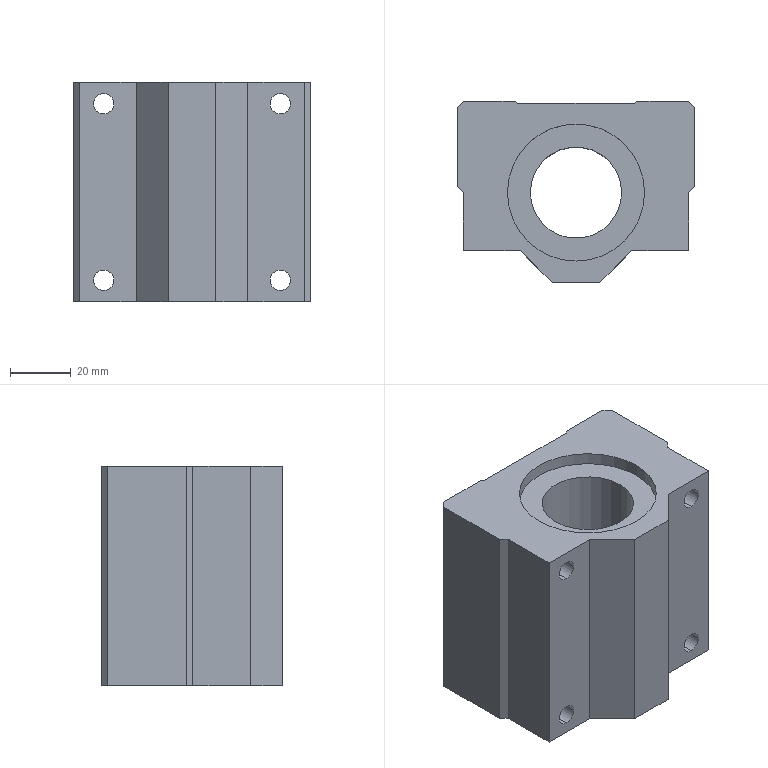Part | SolidWorks | features MBimport 1 | 1 solid | 44 faces | box 78 x 59.5 x 72 mm | volume 221969 mm3 | plane 22 | cylinder 14 | cone 8 | commonest cylinder face diameters 6.647 x8 45 x4 30 x2
STEP:
#1=CARTESIAN_POINT('',(-29.,29.324,-68.323));
#2=VERTEX_POINT('',#1);
#3=CARTESIAN_POINT('',(-29.,29.324,-61.676));
#4=VERTEX_POINT('',#3);
#5=CARTESIAN_POINT('',(-29.,29.324,-65.));
#6=DIRECTION('',(0.,1.,0.));
#7=DIRECTION('',(0.,0.,1.));
#8=AXIS2_PLACEMENT_3D('',#5,#6,#7);
#9=CIRCLE('',#8,3.323);
#10=EDGE_CURVE('',#2,#4,#9,.T.);
#11=ORIENTED_EDGE('',*,*,#10,.F.);
#12=CARTESIAN_POINT('',(-29.,30.,-69.));
#13=VERTEX_POINT('',#12);
#14=CARTESIAN_POINT('',(-29.,29.324,-68.323));
#15=DIRECTION('',(0.,0.7071,-0.7071));
#16=VECTOR('',#15,1000.);
#17=LINE('',#14,#16);
#18=EDGE_CURVE('',#2,#13,#17,.T.);
#19=ORIENTED_EDGE('',*,*,#18,.T.);
#20=CARTESIAN_POINT('',(-29.,30.,-61.));
#21=VERTEX_POINT('',#20);
#22=CARTESIAN_POINT('',(-29.,30.,-65.));
#23=DIRECTION('',(0.,1.,0.));
#24=DIRECTION('',(0.,0.,1.));
#25=AXIS2_PLACEMENT_3D('',#22,#23,#24);
#26=CIRCLE('',#25,4.);
#27=EDGE_CURVE('',#13,#21,#26,.T.);
#28=ORIENTED_EDGE('',*,*,#27,.T.);
#29=CARTESIAN_POINT('',(-29.,29.324,-61.676));
#30=DIRECTION('',(0.,0.7071,0.7071));
#31=VECTOR('',#30,1000.);
#32=LINE('',#29,#31);
#33=EDGE_CURVE('',#4,#21,#32,.T.);
#34=ORIENTED_EDGE('',*,*,#33,.F.);
#35=EDGE_LOOP('',(#11,#19,#28,#34));
#36=FACE_OUTER_BOUND('',#35,.T.);
#37=CARTESIAN_POINT('',(-29.,29.324,-65.));
#38=DIRECTION('',(0.,1.,0.));
#39=DIRECTION('',(0.,0.,1.));
#40=AXIS2_PLACEMENT_3D('',#37,#38,#39);
#41=CONICAL_SURFACE('',#40,3.323,0.7854);
#42=ADVANCED_FACE('',(#36),#41,.F.);
#43=CARTESIAN_POINT('',(-29.,29.324,-65.));
#44=DIRECTION('',(0.,1.,0.));
#45=DIRECTION('',(0.,0.,1.));
#46=AXIS2_PLACEMENT_3D('',#43,#44,#45);
#47=CIRCLE('',#46,3.323);
#48=EDGE_CURVE('',#4,#2,#47,.T.);
#49=ORIENTED_EDGE('',*,*,#48,.T.);
#50=CARTESIAN_POINT('',(-29.,-19.,-68.324));
#51=VERTEX_POINT('',#50);
#52=CARTESIAN_POINT('',(-29.,30.,-68.323));
#53=DIRECTION('',(0.,-1.,0.));
#54=VECTOR('',#53,1000.);
#55=LINE('',#52,#54);
#56=EDGE_CURVE('',#2,#51,#55,.T.);
#57=ORIENTED_EDGE('',*,*,#56,.T.);
#58=CARTESIAN_POINT('',(-29.,-19.,-61.677));
#59=VERTEX_POINT('',#58);
#60=CARTESIAN_POINT('',(-29.,-19.,-65.));
#61=DIRECTION('',(0.,1.,0.));
#62=DIRECTION('',(0.,0.,1.));
#63=AXIS2_PLACEMENT_3D('',#60,#61,#62);
#64=CIRCLE('',#63,3.323);
#65=EDGE_CURVE('',#59,#51,#64,.T.);
#66=ORIENTED_EDGE('',*,*,#65,.F.);
#67=CARTESIAN_POINT('',(-29.,30.,-61.676));
#68=DIRECTION('',(0.,-1.,0.));
#69=VECTOR('',#68,1000.);
#70=LINE('',#67,#69);
#71=EDGE_CURVE('',#4,#59,#70,.T.);
#72=ORIENTED_EDGE('',*,*,#71,.F.);
#73=EDGE_LOOP('',(#49,#57,#66,#72));
#74=FACE_OUTER_BOUND('',#73,.T.);
#75=CARTESIAN_POINT('',(-29.,30.,-65.));
#76=DIRECTION('',(0.,-1.,0.));
#77=DIRECTION('',(0.,0.,1.));
#78=AXIS2_PLACEMENT_3D('',#75,#76,#77);
#79=CYLINDRICAL_SURFACE('',#78,3.323);
#80=ADVANCED_FACE('',(#74),#79,.F.);
#81=CARTESIAN_POINT('',(29.,-19.,-68.324));
#82=VERTEX_POINT('',#81);
#83=CARTESIAN_POINT('',(29.,-19.,-61.677));
#84=VERTEX_POINT('',#83);
#85=CARTESIAN_POINT('',(29.,-19.,-65.));
#86=DIRECTION('',(0.,-1.,0.));
#87=DIRECTION('',(0.,0.,-1.));
#88=AXIS2_PLACEMENT_3D('',#85,#86,#87);
#89=CIRCLE('',#88,3.323);
#90=EDGE_CURVE('',#82,#84,#89,.T.);
#91=ORIENTED_EDGE('',*,*,#90,.T.);
#92=CARTESIAN_POINT('',(29.,29.324,-61.677));
#93=VERTEX_POINT('',#92);
#94=CARTESIAN_POINT('',(29.,-19.,-61.677));
#95=DIRECTION('',(0.,1.,0.));
#96=VECTOR('',#95,1000.);
#97=LINE('',#94,#96);
#98=EDGE_CURVE('',#84,#93,#97,.T.);
#99=ORIENTED_EDGE('',*,*,#98,.T.);
#100=CARTESIAN_POINT('',(29.,29.324,-68.324));
#101=VERTEX_POINT('',#100);
#102=CARTESIAN_POINT('',(29.,29.324,-65.));
#103=DIRECTION('',(0.,-1.,0.));
#104=DIRECTION('',(0.,0.,-1.));
#105=AXIS2_PLACEMENT_3D('',#102,#103,#104);
#106=CIRCLE('',#105,3.323);
#107=EDGE_CURVE('',#101,#93,#106,.T.);
#108=ORIENTED_EDGE('',*,*,#107,.F.);
#109=CARTESIAN_POINT('',(29.,-19.,-68.324));
#110=DIRECTION('',(0.,1.,0.));
#111=VECTOR('',#110,1000.);
#112=LINE('',#109,#111);
#113=EDGE_CURVE('',#82,#101,#112,.T.);
#114=ORIENTED_EDGE('',*,*,#113,.F.);
#115=EDGE_LOOP('',(#91,#99,#108,#114));
#116=FACE_OUTER_BOUND('',#115,.T.);
#117=CARTESIAN_POINT('',(29.,-19.,-65.));
#118=DIRECTION('',(0.,1.,0.));
#119=DIRECTION('',(0.,0.,-1.));
#120=AXIS2_PLACEMENT_3D('',#117,#118,#119);
#121=CYLINDRICAL_SURFACE('',#120,3.323);
#122=ADVANCED_FACE('',(#116),#121,.F.);
#123=CARTESIAN_POINT('',(29.,29.324,-65.));
#124=DIRECTION('',(0.,-1.,0.));
#125=DIRECTION('',(0.,0.,-1.));
#126=AXIS2_PLACEMENT_3D('',#123,#124,#125);
#127=CIRCLE('',#126,3.323);
#128=EDGE_CURVE('',#93,#101,#127,.T.);
#129=ORIENTED_EDGE('',*,*,#128,.T.);
#130=CARTESIAN_POINT('',(29.,30.,-69.));
#131=VERTEX_POINT('',#130);
#132=CARTESIAN_POINT('',(29.,30.,-69.));
#133=DIRECTION('',(0.,0.7071,-0.7071));
#134=VECTOR('',#133,1000.);
#135=LINE('',#132,#134);
#136=EDGE_CURVE('',#101,#131,#135,.T.);
#137=ORIENTED_EDGE('',*,*,#136,.T.);
#138=CARTESIAN_POINT('',(29.,30.,-61.));
#139=VERTEX_POINT('',#138);
#140=CARTESIAN_POINT('',(29.,30.,-65.));
#141=DIRECTION('',(0.,-1.,0.));
#142=DIRECTION('',(0.,0.,-1.));
#143=AXIS2_PLACEMENT_3D('',#140,#141,#142);
#144=CIRCLE('',#143,4.);
#145=EDGE_CURVE('',#139,#131,#144,.T.);
#146=ORIENTED_EDGE('',*,*,#145,.F.);
#147=CARTESIAN_POINT('',(29.,30.,-61.));
#148=DIRECTION('',(0.,0.7071,0.7071));
#149=VECTOR('',#148,1000.);
#150=LINE('',#147,#149);
#151=EDGE_CURVE('',#93,#139,#150,.T.);
#152=ORIENTED_EDGE('',*,*,#151,.F.);
#153=EDGE_LOOP('',(#129,#137,#146,#152));
#154=FACE_OUTER_BOUND('',#153,.T.);
#155=CARTESIAN_POINT('',(29.,30.,-65.));
#156=DIRECTION('',(0.,1.,0.));
#157=DIRECTION('',(0.,0.,1.));
#158=AXIS2_PLACEMENT_3D('',#155,#156,#157);
#159=CONICAL_SURFACE('',#158,4.,0.7854);
#160=ADVANCED_FACE('',(#154),#159,.F.);
#161=CARTESIAN_POINT('',(-29.,29.324,-10.323));
#162=VERTEX_POINT('',#161);
#163=CARTESIAN_POINT('',(-29.,29.324,-3.676));
#164=VERTEX_POINT('',#163);
#165=CARTESIAN_POINT('',(-29.,29.324,-7.));
#166=DIRECTION('',(0.,1.,0.));
#167=DIRECTION('',(0.,0.,1.));
#168=AXIS2_PLACEMENT_3D('',#165,#166,#167);
#169=CIRCLE('',#168,3.323);
#170=EDGE_CURVE('',#162,#164,#169,.T.);
#171=ORIENTED_EDGE('',*,*,#170,.F.);
#172=CARTESIAN_POINT('',(-29.,30.,-11.));
#173=VERTEX_POINT('',#172);
#174=CARTESIAN_POINT('',(-29.,29.324,-10.323));
#175=DIRECTION('',(0.,0.7071,-0.7071));
#176=VECTOR('',#175,1000.);
#177=LINE('',#174,#176);
#178=EDGE_CURVE('',#162,#173,#177,.T.);
#179=ORIENTED_EDGE('',*,*,#178,.T.);
#180=CARTESIAN_POINT('',(-29.,30.,-3.));
#181=VERTEX_POINT('',#180);
#182=CARTESIAN_POINT('',(-29.,30.,-7.));
#183=DIRECTION('',(0.,1.,0.));
#184=DIRECTION('',(0.,0.,1.));
#185=AXIS2_PLACEMENT_3D('',#182,#183,#184);
#186=CIRCLE('',#185,4.);
#187=EDGE_CURVE('',#173,#181,#186,.T.);
#188=ORIENTED_EDGE('',*,*,#187,.T.);
#189=CARTESIAN_POINT('',(-29.,29.324,-3.676));
#190=DIRECTION('',(0.,0.7071,0.7071));
#191=VECTOR('',#190,1000.);
#192=LINE('',#189,#191);
#193=EDGE_CURVE('',#164,#181,#192,.T.);
#194=ORIENTED_EDGE('',*,*,#193,.F.);
#195=EDGE_LOOP('',(#171,#179,#188,#194));
#196=FACE_OUTER_BOUND('',#195,.T.);
#197=CARTESIAN_POINT('',(-29.,29.324,-7.));
#198=DIRECTION('',(0.,1.,0.));
#199=DIRECTION('',(0.,0.,1.));
#200=AXIS2_PLACEMENT_3D('',#197,#198,#199);
#201=CONICAL_SURFACE('',#200,3.323,0.7854);
#202=ADVANCED_FACE('',(#196),#201,.F.);
#203=CARTESIAN_POINT('',(-22.5,0.,-72.));
#204=VERTEX_POINT('',#203);
#205=CARTESIAN_POINT('',(22.5,0.,-72.));
#206=VERTEX_POINT('',#205);
#207=CARTESIAN_POINT('',(0.,0.,-72.));
#208=DIRECTION('',(0.,0.,-1.));
#209=DIRECTION('',(-1.,0.,0.));
#210=AXIS2_PLACEMENT_3D('',#207,#208,#209);
#211=CIRCLE('',#210,22.5);
#212=EDGE_CURVE('',#204,#206,#211,.T.);
#213=ORIENTED_EDGE('',*,*,#212,.T.);
#214=CARTESIAN_POINT('',(22.5,0.,-68.));
#215=VERTEX_POINT('',#214);
#216=CARTESIAN_POINT('',(22.5,0.,-72.));
#217=DIRECTION('',(0.,0.,1.));
#218=VECTOR('',#217,1000.);
#219=LINE('',#216,#218);
#220=EDGE_CURVE('',#206,#215,#219,.T.);
#221=ORIENTED_EDGE('',*,*,#220,.T.);
#222=CARTESIAN_POINT('',(-22.5,0.,-68.));
#223=VERTEX_POINT('',#222);
#224=CARTESIAN_POINT('',(0.,0.,-68.));
#225=DIRECTION('',(0.,0.,-1.));
#226=DIRECTION('',(-1.,0.,0.));
#227=AXIS2_PLACEMENT_3D('',#224,#225,#226);
#228=CIRCLE('',#227,22.5);
#229=EDGE_CURVE('',#223,#215,#228,.T.);
#230=ORIENTED_EDGE('',*,*,#229,.F.);
#231=CARTESIAN_POINT('',(-22.5,0.,-72.));
#232=DIRECTION('',(0.,0.,1.));
#233=VECTOR('',#232,1000.);
#234=LINE('',#231,#233);
#235=EDGE_CURVE('',#204,#223,#234,.T.);
#236=ORIENTED_EDGE('',*,*,#235,.F.);
#237=EDGE_LOOP('',(#213,#221,#230,#236));
#238=FACE_OUTER_BOUND('',#237,.T.);
#239=CARTESIAN_POINT('',(0.,0.,-72.));
#240=DIRECTION('',(0.,0.,1.));
#241=DIRECTION('',(-1.,0.,0.));
#242=AXIS2_PLACEMENT_3D('',#239,#240,#241);
#243=CYLINDRICAL_SURFACE('',#242,22.5);
#244=ADVANCED_FACE('',(#238),#243,.F.);
#245=CARTESIAN_POINT('',(29.,29.324,-3.677));
#246=VERTEX_POINT('',#245);
#247=CARTESIAN_POINT('',(29.,29.324,-10.323));
#248=VERTEX_POINT('',#247);
#249=CARTESIAN_POINT('',(29.,29.324,-7.));
#250=DIRECTION('',(0.,-1.,0.));
#251=DIRECTION('',(0.,0.,-1.));
#252=AXIS2_PLACEMENT_3D('',#249,#250,#251);
#253=CIRCLE('',#252,3.323);
#254=EDGE_CURVE('',#246,#248,#253,.T.);
#255=ORIENTED_EDGE('',*,*,#254,.T.);
#256=CARTESIAN_POINT('',(29.,30.,-11.));
#257=VERTEX_POINT('',#256);
#258=CARTESIAN_POINT('',(29.,30.,-11.));
#259=DIRECTION('',(0.,0.7071,-0.7071));
#260=VECTOR('',#259,1000.);
#261=LINE('',#258,#260);
#262=EDGE_CURVE('',#248,#257,#261,.T.);
#263=ORIENTED_EDGE('',*,*,#262,.T.);
#264=CARTESIAN_POINT('',(29.,30.,-3.));
#265=VERTEX_POINT('',#264);
#266=CARTESIAN_POINT('',(29.,30.,-7.));
#267=DIRECTION('',(0.,-1.,0.));
#268=DIRECTION('',(0.,0.,-1.));
#269=AXIS2_PLACEMENT_3D('',#266,#267,#268);
#270=CIRCLE('',#269,4.);
#271=EDGE_CURVE('',#265,#257,#270,.T.);
#272=ORIENTED_EDGE('',*,*,#271,.F.);
#273=CARTESIAN_POINT('',(29.,30.,-3.));
#274=DIRECTION('',(0.,0.7071,0.7071));
#275=VECTOR('',#274,1000.);
#276=LINE('',#273,#275);
#277=EDGE_CURVE('',#246,#265,#276,.T.);
#278=ORIENTED_EDGE('',*,*,#277,.F.);
#279=EDGE_LOOP('',(#255,#263,#272,#278));
#280=FACE_OUTER_BOUND('',#279,.T.);
#281=CARTESIAN_POINT('',(29.,30.,-7.));
#282=DIRECTION('',(0.,1.,0.));
#283=DIRECTION('',(0.,0.,1.));
#284=AXIS2_PLACEMENT_3D('',#281,#282,#283);
#285=CONICAL_SURFACE('',#284,4.,0.7854);
#286=ADVANCED_FACE('',(#280),#285,.F.);
#287=CARTESIAN_POINT('',(-29.,29.324,-7.));
#288=DIRECTION('',(0.,1.,0.));
#289=DIRECTION('',(0.,0.,1.));
#290=AXIS2_PLACEMENT_3D('',#287,#288,#289);
#291=CIRCLE('',#290,3.323);
#292=EDGE_CURVE('',#164,#162,#291,.T.);
#293=ORIENTED_EDGE('',*,*,#292,.T.);
#294=CARTESIAN_POINT('',(-29.,-19.,-10.324));
#295=VERTEX_POINT('',#294);
#296=CARTESIAN_POINT('',(-29.,30.,-10.323));
#297=DIRECTION('',(0.,-1.,0.));
#298=VECTOR('',#297,1000.);
#299=LINE('',#296,#298);
#300=EDGE_CURVE('',#162,#295,#299,.T.);
#301=ORIENTED_EDGE('',*,*,#300,.T.);
#302=CARTESIAN_POINT('',(-29.,-19.,-3.677));
#303=VERTEX_POINT('',#302);
#304=CARTESIAN_POINT('',(-29.,-19.,-7.));
#305=DIRECTION('',(0.,1.,0.));
#306=DIRECTION('',(0.,0.,1.));
#307=AXIS2_PLACEMENT_3D('',#304,#305,#306);
#308=CIRCLE('',#307,3.323);
#309=EDGE_CURVE('',#303,#295,#308,.T.);
#310=ORIENTED_EDGE('',*,*,#309,.F.);
#311=CARTESIAN_POINT('',(-29.,30.,-3.676));
#312=DIRECTION('',(0.,-1.,0.));
#313=VECTOR('',#312,1000.);
#314=LINE('',#311,#313);
#315=EDGE_CURVE('',#164,#303,#314,.T.);
#316=ORIENTED_EDGE('',*,*,#315,.F.);
#317=EDGE_LOOP('',(#293,#301,#310,#316));
#318=FACE_OUTER_BOUND('',#317,.T.);
#319=CARTESIAN_POINT('',(-29.,30.,-7.));
#320=DIRECTION('',(0.,-1.,0.));
#321=DIRECTION('',(0.,0.,1.));
#322=AXIS2_PLACEMENT_3D('',#319,#320,#321);
#323=CYLINDRICAL_SURFACE('',#322,3.323);
#324=ADVANCED_FACE('',(#318),#323,.F.);
#325=CARTESIAN_POINT('',(29.,-19.,-10.324));
#326=VERTEX_POINT('',#325);
#327=CARTESIAN_POINT('',(29.,-19.,-3.677));
#328=VERTEX_POINT('',#327);
#329=CARTESIAN_POINT('',(29.,-19.,-7.));
#330=DIRECTION('',(0.,-1.,0.));
#331=DIRECTION('',(0.,0.,-1.));
#332=AXIS2_PLACEMENT_3D('',#329,#330,#331);
#333=CIRCLE('',#332,3.323);
#334=EDGE_CURVE('',#326,#328,#333,.T.);
#335=ORIENTED_EDGE('',*,*,#334,.T.);
#336=CARTESIAN_POINT('',(29.,-19.,-3.677));
#337=DIRECTION('',(0.,1.,0.));
#338=VECTOR('',#337,1000.);
#339=LINE('',#336,#338);
#340=EDGE_CURVE('',#328,#246,#339,.T.);
#341=ORIENTED_EDGE('',*,*,#340,.T.);
#342=CARTESIAN_POINT('',(29.,29.324,-7.));
#343=DIRECTION('',(0.,-1.,0.));
#344=DIRECTION('',(0.,0.,-1.));
#345=AXIS2_PLACEMENT_3D('',#342,#343,#344);
#346=CIRCLE('',#345,3.323);
#347=EDGE_CURVE('',#248,#246,#346,.T.);
#348=ORIENTED_EDGE('',*,*,#347,.F.);
#349=CARTESIAN_POINT('',(29.,-19.,-10.324));
#350=DIRECTION('',(0.,1.,0.));
#351=VECTOR('',#350,1000.);
#352=LINE('',#349,#351);
#353=EDGE_CURVE('',#326,#248,#352,.T.);
#354=ORIENTED_EDGE('',*,*,#353,.F.);
#355=EDGE_LOOP('',(#335,#341,#348,#354));
#356=FACE_OUTER_BOUND('',#355,.T.);
#357=CARTESIAN_POINT('',(29.,-19.,-7.));
#358=DIRECTION('',(0.,1.,0.));
#359=DIRECTION('',(0.,0.,-1.));
#360=AXIS2_PLACEMENT_3D('',#357,#358,#359);
#361=CYLINDRICAL_SURFACE('',#360,3.323);
#362=ADVANCED_FACE('',(#356),#361,.F.);
#363=CARTESIAN_POINT('',(-15.,0.,-68.));
#364=VERTEX_POINT('',#363);
#365=CARTESIAN_POINT('',(15.,0.,-68.));
#366=VERTEX_POINT('',#365);
#367=CARTESIAN_POINT('',(0.,0.,-68.));
#368=DIRECTION('',(0.,0.,-1.));
#369=DIRECTION('',(-1.,0.,0.));
#370=AXIS2_PLACEMENT_3D('',#367,#368,#369);
#371=CIRCLE('',#370,15.);
#372=EDGE_CURVE('',#364,#366,#371,.T.);
#373=ORIENTED_EDGE('',*,*,#372,.T.);
#374=CARTESIAN_POINT('',(15.,0.,-4.));
#375=VERTEX_POINT('',#374);
#376=CARTESIAN_POINT('',(15.,0.,-72.));
#377=DIRECTION('',(0.,0.,1.));
#378=VECTOR('',#377,1000.);
#379=LINE('',#376,#378);
#380=EDGE_CURVE('',#366,#375,#379,.T.);
#381=ORIENTED_EDGE('',*,*,#380,.T.);
#382=CARTESIAN_POINT('',(-15.,0.,-4.));
#383=VERTEX_POINT('',#382);
#384=CARTESIAN_POINT('',(0.,0.,-4.));
#385=DIRECTION('',(0.,0.,-1.));
#386=DIRECTION('',(-1.,0.,0.));
#387=AXIS2_PLACEMENT_3D('',#384,#385,#386);
#388=CIRCLE('',#387,15.);
#389=EDGE_CURVE('',#383,#375,#388,.T.);
#390=ORIENTED_EDGE('',*,*,#389,.F.);
#391=CARTESIAN_POINT('',(-15.,0.,-72.));
#392=DIRECTION('',(0.,0.,1.));
#393=VECTOR('',#392,1000.);
#394=LINE('',#391,#393);
#395=EDGE_CURVE('',#364,#383,#394,.T.);
#396=ORIENTED_EDGE('',*,*,#395,.F.);
#397=EDGE_LOOP('',(#373,#381,#390,#396));
#398=FACE_OUTER_BOUND('',#397,.T.);
#399=CARTESIAN_POINT('',(0.,0.,-72.));
#400=DIRECTION('',(0.,0.,1.));
#401=DIRECTION('',(-1.,0.,0.));
#402=AXIS2_PLACEMENT_3D('',#399,#400,#401);
#403=CYLINDRICAL_SURFACE('',#402,15.);
#404=ADVANCED_FACE('',(#398),#403,.F.);
#405=CARTESIAN_POINT('',(-22.5,0.,-4.));
#406=VERTEX_POINT('',#405);
#407=CARTESIAN_POINT('',(22.5,0.,-4.));
#408=VERTEX_POINT('',#407);
#409=CARTESIAN_POINT('',(0.,0.,-4.));
#410=DIRECTION('',(0.,0.,-1.));
#411=DIRECTION('',(-1.,0.,0.));
#412=AXIS2_PLACEMENT_3D('',#409,#410,#411);
#413=CIRCLE('',#412,22.5);
#414=EDGE_CURVE('',#406,#408,#413,.T.);
#415=ORIENTED_EDGE('',*,*,#414,.T.);
#416=CARTESIAN_POINT('',(22.5,0.,0.));
#417=VERTEX_POINT('',#416);
#418=CARTESIAN_POINT('',(22.5,0.,-72.));
#419=DIRECTION('',(0.,0.,1.));
#420=VECTOR('',#419,1000.);
#421=LINE('',#418,#420);
#422=EDGE_CURVE('',#408,#417,#421,.T.);
#423=ORIENTED_EDGE('',*,*,#422,.T.);
#424=CARTESIAN_POINT('',(-22.5,0.,0.));
#425=VERTEX_POINT('',#424);
#426=CARTESIAN_POINT('',(0.,0.,0.));
#427=DIRECTION('',(0.,0.,-1.));
#428=DIRECTION('',(-1.,0.,0.));
#429=AXIS2_PLACEMENT_3D('',#426,#427,#428);
#430=CIRCLE('',#429,22.5);
#431=EDGE_CURVE('',#425,#417,#430,.T.);
#432=ORIENTED_EDGE('',*,*,#431,.F.);
#433=CARTESIAN_POINT('',(-22.5,0.,-72.));
#434=DIRECTION('',(0.,0.,1.));
#435=VECTOR('',#434,1000.);
#436=LINE('',#433,#435);
#437=EDGE_CURVE('',#406,#425,#436,.T.);
#438=ORIENTED_EDGE('',*,*,#437,.F.);
#439=EDGE_LOOP('',(#415,#423,#432,#438));
#440=FACE_OUTER_BOUND('',#439,.T.);
#441=CARTESIAN_POINT('',(0.,0.,-72.));
#442=DIRECTION('',(0.,0.,1.));
#443=DIRECTION('',(-1.,0.,0.));
#444=AXIS2_PLACEMENT_3D('',#441,#442,#443);
#445=CYLINDRICAL_SURFACE('',#444,22.5);
#446=ADVANCED_FACE('',(#440),#445,.F.);
#447=CARTESIAN_POINT('',(-37.,-19.,0.));
#448=VERTEX_POINT('',#447);
#449=CARTESIAN_POINT('',(-18.3,-19.,0.));
#450=VERTEX_POINT('',#449);
#451=CARTESIAN_POINT('',(-37.,-19.,0.));
#452=DIRECTION('',(1.,0.,0.));
#453=VECTOR('',#452,1000.);
#454=LINE('',#451,#453);
#455=EDGE_CURVE('',#448,#450,#454,.T.);
#456=ORIENTED_EDGE('',*,*,#455,.F.);
#457=CARTESIAN_POINT('',(-37.,-19.,-72.));
#458=VERTEX_POINT('',#457);
#459=CARTESIAN_POINT('',(-37.,-19.,-72.));
#460=DIRECTION('',(0.,0.,1.));
#461=VECTOR('',#460,1000.);
#462=LINE('',#459,#461);
#463=EDGE_CURVE('',#458,#448,#462,.T.);
#464=ORIENTED_EDGE('',*,*,#463,.F.);
#465=CARTESIAN_POINT('',(-18.3,-19.,-72.));
#466=VERTEX_POINT('',#465);
#467=CARTESIAN_POINT('',(-37.,-19.,-72.));
#468=DIRECTION('',(1.,0.,0.));
#469=VECTOR('',#468,1000.);
#470=LINE('',#467,#469);
#471=EDGE_CURVE('',#458,#466,#470,.T.);
#472=ORIENTED_EDGE('',*,*,#471,.T.);
#473=CARTESIAN_POINT('',(-18.3,-19.,-72.));
#474=DIRECTION('',(0.,0.,1.));
#475=VECTOR('',#474,1000.);
#476=LINE('',#473,#475);
#477=EDGE_CURVE('',#466,#450,#476,.T.);
#478=ORIENTED_EDGE('',*,*,#477,.T.);
#479=EDGE_LOOP('',(#456,#464,#472,#478));
#480=FACE_OUTER_BOUND('',#479,.T.);
#481=ORIENTED_EDGE('',*,*,#309,.T.);
#482=CARTESIAN_POINT('',(-29.,-19.,-7.));
#483=DIRECTION('',(0.,1.,0.));
#484=DIRECTION('',(0.,0.,1.));
#485=AXIS2_PLACEMENT_3D('',#482,#483,#484);
#486=CIRCLE('',#485,3.323);
#487=EDGE_CURVE('',#295,#303,#486,.T.);
#488=ORIENTED_EDGE('',*,*,#487,.T.);
#489=EDGE_LOOP('',(#481,#488));
#490=FACE_BOUND('',#489,.T.);
#491=ORIENTED_EDGE('',*,*,#65,.T.);
#492=CARTESIAN_POINT('',(-29.,-19.,-65.));
#493=DIRECTION('',(0.,1.,0.));
#494=DIRECTION('',(0.,0.,1.));
#495=AXIS2_PLACEMENT_3D('',#492,#493,#494);
#496=CIRCLE('',#495,3.323);
#497=EDGE_CURVE('',#51,#59,#496,.T.);
#498=ORIENTED_EDGE('',*,*,#497,.T.);
#499=EDGE_LOOP('',(#491,#498));
#500=FACE_BOUND('',#499,.T.);
#501=CARTESIAN_POINT('',(-37.,-19.,-72.));
#502=DIRECTION('',(0.,-1.,0.));
#503=DIRECTION('',(0.,0.,-1.));
#504=AXIS2_PLACEMENT_3D('',#501,#502,#503);
#505=PLANE('',#504);
#506=ADVANCED_FACE('',(#480,#490,#500),#505,.T.);
#507=CARTESIAN_POINT('',(-39.,28.,0.));
#508=VERTEX_POINT('',#507);
#509=CARTESIAN_POINT('',(-39.,2.,0.));
#510=VERTEX_POINT('',#509);
#511=CARTESIAN_POINT('',(-39.,28.,0.));
#512=DIRECTION('',(0.,-1.,0.));
#513=VECTOR('',#512,1000.);
#514=LINE('',#511,#513);
#515=EDGE_CURVE('',#508,#510,#514,.T.);
#516=ORIENTED_EDGE('',*,*,#515,.F.);
#517=CARTESIAN_POINT('',(-39.,28.,-72.));
#518=VERTEX_POINT('',#517);
#519=CARTESIAN_POINT('',(-39.,28.,-72.));
#520=DIRECTION('',(0.,0.,1.));
#521=VECTOR('',#520,1000.);
#522=LINE('',#519,#521);
#523=EDGE_CURVE('',#518,#508,#522,.T.);
#524=ORIENTED_EDGE('',*,*,#523,.F.);
#525=CARTESIAN_POINT('',(-39.,2.,-72.));
#526=VERTEX_POINT('',#525);
#527=CARTESIAN_POINT('',(-39.,28.,-72.));
#528=DIRECTION('',(0.,-1.,0.));
#529=VECTOR('',#528,1000.);
#530=LINE('',#527,#529);
#531=EDGE_CURVE('',#518,#526,#530,.T.);
#532=ORIENTED_EDGE('',*,*,#531,.T.);
#533=CARTESIAN_POINT('',(-39.,2.,-72.));
#534=DIRECTION('',(0.,0.,1.));
#535=VECTOR('',#534,1000.);
#536=LINE('',#533,#535);
#537=EDGE_CURVE('',#526,#510,#536,.T.);
#538=ORIENTED_EDGE('',*,*,#537,.T.);
#539=EDGE_LOOP('',(#516,#524,#532,#538));
#540=FACE_OUTER_BOUND('',#539,.T.);
#541=CARTESIAN_POINT('',(-39.,28.,-72.));
#542=DIRECTION('',(-1.,0.,0.));
#543=DIRECTION('',(0.,0.,1.));
#544=AXIS2_PLACEMENT_3D('',#541,#542,#543);
#545=PLANE('',#544);
#546=ADVANCED_FACE('',(#540),#545,.T.);
#547=CARTESIAN_POINT('',(-19.95,30.,0.));
#548=VERTEX_POINT('',#547);
#549=CARTESIAN_POINT('',(-37.,30.,0.));
#550=VERTEX_POINT('',#549);
#551=CARTESIAN_POINT('',(-19.95,30.,0.));
#552=DIRECTION('',(-1.,0.,0.));
#553=VECTOR('',#552,1000.);
#554=LINE('',#551,#553);
#555=EDGE_CURVE('',#548,#550,#554,.T.);
#556=ORIENTED_EDGE('',*,*,#555,.F.);
#557=CARTESIAN_POINT('',(-19.95,30.,-72.));
#558=VERTEX_POINT('',#557);
#559=CARTESIAN_POINT('',(-19.95,30.,-72.));
#560=DIRECTION('',(0.,0.,1.));
#561=VECTOR('',#560,1000.);
#562=LINE('',#559,#561);
#563=EDGE_CURVE('',#558,#548,#562,.T.);
#564=ORIENTED_EDGE('',*,*,#563,.F.);
#565=CARTESIAN_POINT('',(-37.,30.,-72.));
#566=VERTEX_POINT('',#565);
#567=CARTESIAN_POINT('',(-19.95,30.,-72.));
#568=DIRECTION('',(-1.,0.,0.));
#569=VECTOR('',#568,1000.);
#570=LINE('',#567,#569);
#571=EDGE_CURVE('',#558,#566,#570,.T.);
#572=ORIENTED_EDGE('',*,*,#571,.T.);
#573=CARTESIAN_POINT('',(-37.,30.,-72.));
#574=DIRECTION('',(0.,0.,1.));
#575=VECTOR('',#574,1000.);
#576=LINE('',#573,#575);
#577=EDGE_CURVE('',#566,#550,#576,.T.);
#578=ORIENTED_EDGE('',*,*,#577,.T.);
#579=EDGE_LOOP('',(#556,#564,#572,#578));
#580=FACE_OUTER_BOUND('',#579,.T.);
#581=CARTESIAN_POINT('',(-29.,30.,-7.));
#582=DIRECTION('',(0.,1.,0.));
#583=DIRECTION('',(0.,0.,1.));
#584=AXIS2_PLACEMENT_3D('',#581,#582,#583);
#585=CIRCLE('',#584,4.);
#586=EDGE_CURVE('',#181,#173,#585,.T.);
#587=ORIENTED_EDGE('',*,*,#586,.F.);
#588=ORIENTED_EDGE('',*,*,#187,.F.);
#589=EDGE_LOOP('',(#587,#588));
#590=FACE_BOUND('',#589,.T.);
#591=CARTESIAN_POINT('',(-29.,30.,-65.));
#592=DIRECTION('',(0.,1.,0.));
#593=DIRECTION('',(0.,0.,1.));
#594=AXIS2_PLACEMENT_3D('',#591,#592,#593);
#595=CIRCLE('',#594,4.);
#596=EDGE_CURVE('',#21,#13,#595,.T.);
#597=ORIENTED_EDGE('',*,*,#596,.F.);
#598=ORIENTED_EDGE('',*,*,#27,.F.);
#599=EDGE_LOOP('',(#597,#598));
#600=FACE_BOUND('',#599,.T.);
#601=CARTESIAN_POINT('',(-19.95,30.,-72.));
#602=DIRECTION('',(0.,1.,0.));
#603=DIRECTION('',(1.,0.,0.));
#604=AXIS2_PLACEMENT_3D('',#601,#602,#603);
#605=PLANE('',#604);
#606=ADVANCED_FACE('',(#580,#590,#600),#605,.T.);
#607=CARTESIAN_POINT('',(-19.2,29.25,0.));
#608=VERTEX_POINT('',#607);
#609=CARTESIAN_POINT('',(-19.2,29.25,0.));
#610=DIRECTION('',(-0.7071,0.7071,0.));
#611=VECTOR('',#610,1000.);
#612=LINE('',#609,#611);
#613=EDGE_CURVE('',#608,#548,#612,.T.);
#614=ORIENTED_EDGE('',*,*,#613,.F.);
#615=CARTESIAN_POINT('',(-19.2,29.25,-72.));
#616=VERTEX_POINT('',#615);
#617=CARTESIAN_POINT('',(-19.2,29.25,-72.));
#618=DIRECTION('',(0.,0.,1.));
#619=VECTOR('',#618,1000.);
#620=LINE('',#617,#619);
#621=EDGE_CURVE('',#616,#608,#620,.T.);
#622=ORIENTED_EDGE('',*,*,#621,.F.);
#623=CARTESIAN_POINT('',(-19.2,29.25,-72.));
#624=DIRECTION('',(-0.7071,0.7071,0.));
#625=VECTOR('',#624,1000.);
#626=LINE('',#623,#625);
#627=EDGE_CURVE('',#616,#558,#626,.T.);
#628=ORIENTED_EDGE('',*,*,#627,.T.);
#629=ORIENTED_EDGE('',*,*,#563,.T.);
#630=EDGE_LOOP('',(#614,#622,#628,#629));
#631=FACE_OUTER_BOUND('',#630,.T.);
#632=CARTESIAN_POINT('',(-19.2,29.25,-72.));
#633=DIRECTION('',(0.7071,0.7071,0.));
#634=DIRECTION('',(0.,0.,-1.));
#635=AXIS2_PLACEMENT_3D('',#632,#633,#634);
#636=PLANE('',#635);
#637=ADVANCED_FACE('',(#631),#636,.T.);
#638=ORIENTED_EDGE('',*,*,#531,.F.);
#639=CARTESIAN_POINT('',(-37.,30.,-72.));
#640=DIRECTION('',(-0.7071,-0.7071,0.));
#641=VECTOR('',#640,1000.);
#642=LINE('',#639,#641);
#643=EDGE_CURVE('',#566,#518,#642,.T.);
#644=ORIENTED_EDGE('',*,*,#643,.F.);
#645=ORIENTED_EDGE('',*,*,#571,.F.);
#646=ORIENTED_EDGE('',*,*,#627,.F.);
#647=CARTESIAN_POINT('',(19.2,29.25,-72.));
#648=VERTEX_POINT('',#647);
#649=CARTESIAN_POINT('',(19.2,29.25,-72.));
#650=DIRECTION('',(-1.,0.,0.));
#651=VECTOR('',#650,1000.);
#652=LINE('',#649,#651);
#653=EDGE_CURVE('',#648,#616,#652,.T.);
#654=ORIENTED_EDGE('',*,*,#653,.F.);
#655=CARTESIAN_POINT('',(19.95,30.,-72.));
#656=VERTEX_POINT('',#655);
#657=CARTESIAN_POINT('',(19.95,30.,-72.));
#658=DIRECTION('',(-0.7071,-0.7071,0.));
#659=VECTOR('',#658,1000.);
#660=LINE('',#657,#659);
#661=EDGE_CURVE('',#656,#648,#660,.T.);
#662=ORIENTED_EDGE('',*,*,#661,.F.);
#663=CARTESIAN_POINT('',(37.,30.,-72.));
#664=VERTEX_POINT('',#663);
#665=CARTESIAN_POINT('',(37.,30.,-72.));
#666=DIRECTION('',(-1.,0.,0.));
#667=VECTOR('',#666,1000.);
#668=LINE('',#665,#667);
#669=EDGE_CURVE('',#664,#656,#668,.T.);
#670=ORIENTED_EDGE('',*,*,#669,.F.);
#671=CARTESIAN_POINT('',(39.,28.,-72.));
#672=VERTEX_POINT('',#671);
#673=CARTESIAN_POINT('',(39.,28.,-72.));
#674=DIRECTION('',(-0.7071,0.7071,0.));
#675=VECTOR('',#674,1000.);
#676=LINE('',#673,#675);
#677=EDGE_CURVE('',#672,#664,#676,.T.);
#678=ORIENTED_EDGE('',*,*,#677,.F.);
#679=CARTESIAN_POINT('',(39.,2.,-72.));
#680=VERTEX_POINT('',#679);
#681=CARTESIAN_POINT('',(39.,2.,-72.));
#682=DIRECTION('',(0.,1.,0.));
#683=VECTOR('',#682,1000.);
#684=LINE('',#681,#683);
#685=EDGE_CURVE('',#680,#672,#684,.T.);
#686=ORIENTED_EDGE('',*,*,#685,.F.);
#687=CARTESIAN_POINT('',(37.,0.,-72.));
#688=VERTEX_POINT('',#687);
#689=CARTESIAN_POINT('',(37.,0.,-72.));
#690=DIRECTION('',(0.7071,0.7071,0.));
#691=VECTOR('',#690,1000.);
#692=LINE('',#689,#691);
#693=EDGE_CURVE('',#688,#680,#692,.T.);
#694=ORIENTED_EDGE('',*,*,#693,.F.);
#695=CARTESIAN_POINT('',(37.,-19.,-72.));
#696=VERTEX_POINT('',#695);
#697=CARTESIAN_POINT('',(37.,-19.,-72.));
#698=DIRECTION('',(0.,1.,0.));
#699=VECTOR('',#698,1000.);
#700=LINE('',#697,#699);
#701=EDGE_CURVE('',#696,#688,#700,.T.);
#702=ORIENTED_EDGE('',*,*,#701,.F.);
#703=CARTESIAN_POINT('',(18.3,-19.,-72.));
#704=VERTEX_POINT('',#703);
#705=CARTESIAN_POINT('',(18.3,-19.,-72.));
#706=DIRECTION('',(1.,0.,0.));
#707=VECTOR('',#706,1000.);
#708=LINE('',#705,#707);
#709=EDGE_CURVE('',#704,#696,#708,.T.);
#710=ORIENTED_EDGE('',*,*,#709,.F.);
#711=CARTESIAN_POINT('',(7.8,-29.5,-72.));
#712=VERTEX_POINT('',#711);
#713=CARTESIAN_POINT('',(7.8,-29.5,-72.));
#714=DIRECTION('',(0.7071,0.7071,0.));
#715=VECTOR('',#714,1000.);
#716=LINE('',#713,#715);
#717=EDGE_CURVE('',#712,#704,#716,.T.);
#718=ORIENTED_EDGE('',*,*,#717,.F.);
#719=CARTESIAN_POINT('',(-7.8,-29.5,-72.));
#720=VERTEX_POINT('',#719);
#721=CARTESIAN_POINT('',(-7.8,-29.5,-72.));
#722=DIRECTION('',(1.,0.,0.));
#723=VECTOR('',#722,1000.);
#724=LINE('',#721,#723);
#725=EDGE_CURVE('',#720,#712,#724,.T.);
#726=ORIENTED_EDGE('',*,*,#725,.F.);
#727=CARTESIAN_POINT('',(-18.3,-19.,-72.));
#728=DIRECTION('',(0.7071,-0.7071,0.));
#729=VECTOR('',#728,1000.);
#730=LINE('',#727,#729);
#731=EDGE_CURVE('',#466,#720,#730,.T.);
#732=ORIENTED_EDGE('',*,*,#731,.F.);
#733=ORIENTED_EDGE('',*,*,#471,.F.);
#734=CARTESIAN_POINT('',(-37.,0.,-72.));
#735=VERTEX_POINT('',#734);
#736=CARTESIAN_POINT('',(-37.,0.,-72.));
#737=DIRECTION('',(0.,-1.,0.));
#738=VECTOR('',#737,1000.);
#739=LINE('',#736,#738);
#740=EDGE_CURVE('',#735,#458,#739,.T.);
#741=ORIENTED_EDGE('',*,*,#740,.F.);
#742=CARTESIAN_POINT('',(-39.,2.,-72.));
#743=DIRECTION('',(0.7071,-0.7071,0.));
#744=VECTOR('',#743,1000.);
#745=LINE('',#742,#744);
#746=EDGE_CURVE('',#526,#735,#745,.T.);
#747=ORIENTED_EDGE('',*,*,#746,.F.);
#748=EDGE_LOOP('',(#638,#644,#645,#646,#654,#662,#670,#678,#686,#694,#702,#710,#718,#726,#732,#733,#741,#747));
#749=FACE_OUTER_BOUND('',#748,.T.);
#750=ORIENTED_EDGE('',*,*,#212,.F.);
#751=CARTESIAN_POINT('',(0.,0.,-72.));
#752=DIRECTION('',(0.,0.,-1.));
#753=DIRECTION('',(-1.,0.,0.));
#754=AXIS2_PLACEMENT_3D('',#751,#752,#753);
#755=CIRCLE('',#754,22.5);
#756=EDGE_CURVE('',#206,#204,#755,.T.);
#757=ORIENTED_EDGE('',*,*,#756,.F.);
#758=EDGE_LOOP('',(#750,#757));
#759=FACE_BOUND('',#758,.T.);
#760=CARTESIAN_POINT('',(0.,0.,-72.));
#761=DIRECTION('',(0.,0.,1.));
#762=DIRECTION('',(1.,0.,0.));
#763=AXIS2_PLACEMENT_3D('',#760,#761,#762);
#764=PLANE('',#763);
#765=ADVANCED_FACE('',(#749,#759),#764,.F.);
#766=CARTESIAN_POINT('',(-37.,0.,0.));
#767=VERTEX_POINT('',#766);
#768=CARTESIAN_POINT('',(-39.,2.,0.));
#769=DIRECTION('',(0.7071,-0.7071,0.));
#770=VECTOR('',#769,1000.);
#771=LINE('',#768,#770);
#772=EDGE_CURVE('',#510,#767,#771,.T.);
#773=ORIENTED_EDGE('',*,*,#772,.F.);
#774=ORIENTED_EDGE('',*,*,#537,.F.);
#775=ORIENTED_EDGE('',*,*,#746,.T.);
#776=CARTESIAN_POINT('',(-37.,0.,-72.));
#777=DIRECTION('',(0.,0.,1.));
#778=VECTOR('',#777,1000.);
#779=LINE('',#776,#778);
#780=EDGE_CURVE('',#735,#767,#779,.T.);
#781=ORIENTED_EDGE('',*,*,#780,.T.);
#782=EDGE_LOOP('',(#773,#774,#775,#781));
#783=FACE_OUTER_BOUND('',#782,.T.);
#784=CARTESIAN_POINT('',(-39.,2.,-72.));
#785=DIRECTION('',(-0.7071,-0.7071,0.));
#786=DIRECTION('',(-0.7071,0.7071,0.));
#787=AXIS2_PLACEMENT_3D('',#784,#785,#786);
#788=PLANE('',#787);
#789=ADVANCED_FACE('',(#783),#788,.T.);
#790=CARTESIAN_POINT('',(-37.,0.,0.));
#791=DIRECTION('',(0.,-1.,0.));
#792=VECTOR('',#791,1000.);
#793=LINE('',#790,#792);
#794=EDGE_CURVE('',#767,#448,#793,.T.);
#795=ORIENTED_EDGE('',*,*,#794,.F.);
#796=ORIENTED_EDGE('',*,*,#780,.F.);
#797=ORIENTED_EDGE('',*,*,#740,.T.);
#798=ORIENTED_EDGE('',*,*,#463,.T.);
#799=EDGE_LOOP('',(#795,#796,#797,#798));
#800=FACE_OUTER_BOUND('',#799,.T.);
#801=CARTESIAN_POINT('',(-37.,0.,-72.));
#802=DIRECTION('',(-1.,0.,0.));
#803=DIRECTION('',(0.,0.,1.));
#804=AXIS2_PLACEMENT_3D('',#801,#802,#803);
#805=PLANE('',#804);
#806=ADVANCED_FACE('',(#800),#805,.T.);
#807=ORIENTED_EDGE('',*,*,#515,.T.);
#808=ORIENTED_EDGE('',*,*,#772,.T.);
#809=ORIENTED_EDGE('',*,*,#794,.T.);
#810=ORIENTED_EDGE('',*,*,#455,.T.);
#811=CARTESIAN_POINT('',(-7.8,-29.5,0.));
#812=VERTEX_POINT('',#811);
#813=CARTESIAN_POINT('',(-18.3,-19.,0.));
#814=DIRECTION('',(0.7071,-0.7071,0.));
#815=VECTOR('',#814,1000.);
#816=LINE('',#813,#815);
#817=EDGE_CURVE('',#450,#812,#816,.T.);
#818=ORIENTED_EDGE('',*,*,#817,.T.);
#819=CARTESIAN_POINT('',(7.8,-29.5,0.));
#820=VERTEX_POINT('',#819);
#821=CARTESIAN_POINT('',(-7.8,-29.5,0.));
#822=DIRECTION('',(1.,0.,0.));
#823=VECTOR('',#822,1000.);
#824=LINE('',#821,#823);
#825=EDGE_CURVE('',#812,#820,#824,.T.);
#826=ORIENTED_EDGE('',*,*,#825,.T.);
#827=CARTESIAN_POINT('',(18.3,-19.,0.));
#828=VERTEX_POINT('',#827);
#829=CARTESIAN_POINT('',(7.8,-29.5,0.));
#830=DIRECTION('',(0.7071,0.7071,0.));
#831=VECTOR('',#830,1000.);
#832=LINE('',#829,#831);
#833=EDGE_CURVE('',#820,#828,#832,.T.);
#834=ORIENTED_EDGE('',*,*,#833,.T.);
#835=CARTESIAN_POINT('',(37.,-19.,0.));
#836=VERTEX_POINT('',#835);
#837=CARTESIAN_POINT('',(18.3,-19.,0.));
#838=DIRECTION('',(1.,0.,0.));
#839=VECTOR('',#838,1000.);
#840=LINE('',#837,#839);
#841=EDGE_CURVE('',#828,#836,#840,.T.);
#842=ORIENTED_EDGE('',*,*,#841,.T.);
#843=CARTESIAN_POINT('',(37.,0.,0.));
#844=VERTEX_POINT('',#843);
#845=CARTESIAN_POINT('',(37.,-19.,0.));
#846=DIRECTION('',(0.,1.,0.));
#847=VECTOR('',#846,1000.);
#848=LINE('',#845,#847);
#849=EDGE_CURVE('',#836,#844,#848,.T.);
#850=ORIENTED_EDGE('',*,*,#849,.T.);
#851=CARTESIAN_POINT('',(39.,2.,0.));
#852=VERTEX_POINT('',#851);
#853=CARTESIAN_POINT('',(37.,0.,0.));
#854=DIRECTION('',(0.7071,0.7071,0.));
#855=VECTOR('',#854,1000.);
#856=LINE('',#853,#855);
#857=EDGE_CURVE('',#844,#852,#856,.T.);
#858=ORIENTED_EDGE('',*,*,#857,.T.);
#859=CARTESIAN_POINT('',(39.,28.,0.));
#860=VERTEX_POINT('',#859);
#861=CARTESIAN_POINT('',(39.,2.,0.));
#862=DIRECTION('',(0.,1.,0.));
#863=VECTOR('',#862,1000.);
#864=LINE('',#861,#863);
#865=EDGE_CURVE('',#852,#860,#864,.T.);
#866=ORIENTED_EDGE('',*,*,#865,.T.);
#867=CARTESIAN_POINT('',(37.,30.,0.));
#868=VERTEX_POINT('',#867);
#869=CARTESIAN_POINT('',(39.,28.,0.));
#870=DIRECTION('',(-0.7071,0.7071,0.));
#871=VECTOR('',#870,1000.);
#872=LINE('',#869,#871);
#873=EDGE_CURVE('',#860,#868,#872,.T.);
#874=ORIENTED_EDGE('',*,*,#873,.T.);
#875=CARTESIAN_POINT('',(19.95,30.,0.));
#876=VERTEX_POINT('',#875);
#877=CARTESIAN_POINT('',(37.,30.,0.));
#878=DIRECTION('',(-1.,0.,0.));
#879=VECTOR('',#878,1000.);
#880=LINE('',#877,#879);
#881=EDGE_CURVE('',#868,#876,#880,.T.);
#882=ORIENTED_EDGE('',*,*,#881,.T.);
#883=CARTESIAN_POINT('',(19.2,29.25,0.));
#884=VERTEX_POINT('',#883);
#885=CARTESIAN_POINT('',(19.95,30.,0.));
#886=DIRECTION('',(-0.7071,-0.7071,0.));
#887=VECTOR('',#886,1000.);
#888=LINE('',#885,#887);
#889=EDGE_CURVE('',#876,#884,#888,.T.);
#890=ORIENTED_EDGE('',*,*,#889,.T.);
#891=CARTESIAN_POINT('',(19.2,29.25,0.));
#892=DIRECTION('',(-1.,0.,0.));
#893=VECTOR('',#892,1000.);
#894=LINE('',#891,#893);
#895=EDGE_CURVE('',#884,#608,#894,.T.);
#896=ORIENTED_EDGE('',*,*,#895,.T.);
#897=ORIENTED_EDGE('',*,*,#613,.T.);
#898=ORIENTED_EDGE('',*,*,#555,.T.);
#899=CARTESIAN_POINT('',(-37.,30.,0.));
#900=DIRECTION('',(-0.7071,-0.7071,0.));
#901=VECTOR('',#900,1000.);
#902=LINE('',#899,#901);
#903=EDGE_CURVE('',#550,#508,#902,.T.);
#904=ORIENTED_EDGE('',*,*,#903,.T.);
#905=EDGE_LOOP('',(#807,#808,#809,#810,#818,#826,#834,#842,#850,#858,#866,#874,#882,#890,#896,#897,#898,#904));
#906=FACE_OUTER_BOUND('',#905,.T.);
#907=ORIENTED_EDGE('',*,*,#431,.T.);
#908=CARTESIAN_POINT('',(0.,0.,0.));
#909=DIRECTION('',(0.,0.,-1.));
#910=DIRECTION('',(-1.,0.,0.));
#911=AXIS2_PLACEMENT_3D('',#908,#909,#910);
#912=CIRCLE('',#911,22.5);
#913=EDGE_CURVE('',#417,#425,#912,.T.);
#914=ORIENTED_EDGE('',*,*,#913,.T.);
#915=EDGE_LOOP('',(#907,#914));
#916=FACE_BOUND('',#915,.T.);
#917=CARTESIAN_POINT('',(0.,0.,0.));
#918=DIRECTION('',(0.,0.,1.));
#919=DIRECTION('',(1.,0.,0.));
#920=AXIS2_PLACEMENT_3D('',#917,#918,#919);
#921=PLANE('',#920);
#922=ADVANCED_FACE('',(#906,#916),#921,.T.);
#923=ORIENTED_EDGE('',*,*,#895,.F.);
#924=CARTESIAN_POINT('',(19.2,29.25,-72.));
#925=DIRECTION('',(0.,0.,1.));
#926=VECTOR('',#925,1000.);
#927=LINE('',#924,#926);
#928=EDGE_CURVE('',#648,#884,#927,.T.);
#929=ORIENTED_EDGE('',*,*,#928,.F.);
#930=ORIENTED_EDGE('',*,*,#653,.T.);
#931=ORIENTED_EDGE('',*,*,#621,.T.);
#932=EDGE_LOOP('',(#923,#929,#930,#931));
#933=FACE_OUTER_BOUND('',#932,.T.);
#934=CARTESIAN_POINT('',(19.2,29.25,-72.));
#935=DIRECTION('',(0.,1.,0.));
#936=DIRECTION('',(1.,0.,0.));
#937=AXIS2_PLACEMENT_3D('',#934,#935,#936);
#938=PLANE('',#937);
#939=ADVANCED_FACE('',(#933),#938,.T.);
#940=ORIENTED_EDGE('',*,*,#889,.F.);
#941=CARTESIAN_POINT('',(19.95,30.,-72.));
#942=DIRECTION('',(0.,0.,1.));
#943=VECTOR('',#942,1000.);
#944=LINE('',#941,#943);
#945=EDGE_CURVE('',#656,#876,#944,.T.);
#946=ORIENTED_EDGE('',*,*,#945,.F.);
#947=ORIENTED_EDGE('',*,*,#661,.T.);
#948=ORIENTED_EDGE('',*,*,#928,.T.);
#949=EDGE_LOOP('',(#940,#946,#947,#948));
#950=FACE_OUTER_BOUND('',#949,.T.);
#951=CARTESIAN_POINT('',(19.95,30.,-72.));
#952=DIRECTION('',(-0.7071,0.7071,0.));
#953=DIRECTION('',(0.,0.,1.));
#954=AXIS2_PLACEMENT_3D('',#951,#952,#953);
#955=PLANE('',#954);
#956=ADVANCED_FACE('',(#950),#955,.T.);
#957=ORIENTED_EDGE('',*,*,#881,.F.);
#958=CARTESIAN_POINT('',(37.,30.,-72.));
#959=DIRECTION('',(0.,0.,1.));
#960=VECTOR('',#959,1000.);
#961=LINE('',#958,#960);
#962=EDGE_CURVE('',#664,#868,#961,.T.);
#963=ORIENTED_EDGE('',*,*,#962,.F.);
#964=ORIENTED_EDGE('',*,*,#669,.T.);
#965=ORIENTED_EDGE('',*,*,#945,.T.);
#966=EDGE_LOOP('',(#957,#963,#964,#965));
#967=FACE_OUTER_BOUND('',#966,.T.);
#968=ORIENTED_EDGE('',*,*,#271,.T.);
#969=CARTESIAN_POINT('',(29.,30.,-7.));
#970=DIRECTION('',(0.,-1.,0.));
#971=DIRECTION('',(0.,0.,-1.));
#972=AXIS2_PLACEMENT_3D('',#969,#970,#971);
#973=CIRCLE('',#972,4.);
#974=EDGE_CURVE('',#257,#265,#973,.T.);
#975=ORIENTED_EDGE('',*,*,#974,.T.);
#976=EDGE_LOOP('',(#968,#975));
#977=FACE_BOUND('',#976,.T.);
#978=ORIENTED_EDGE('',*,*,#145,.T.);
#979=CARTESIAN_POINT('',(29.,30.,-65.));
#980=DIRECTION('',(0.,-1.,0.));
#981=DIRECTION('',(0.,0.,-1.));
#982=AXIS2_PLACEMENT_3D('',#979,#980,#981);
#983=CIRCLE('',#982,4.);
#984=EDGE_CURVE('',#131,#139,#983,.T.);
#985=ORIENTED_EDGE('',*,*,#984,.T.);
#986=EDGE_LOOP('',(#978,#985));
#987=FACE_BOUND('',#986,.T.);
#988=CARTESIAN_POINT('',(37.,30.,-72.));
#989=DIRECTION('',(0.,1.,0.));
#990=DIRECTION('',(1.,0.,0.));
#991=AXIS2_PLACEMENT_3D('',#988,#989,#990);
#992=PLANE('',#991);
#993=ADVANCED_FACE('',(#967,#977,#987),#992,.T.);
#994=ORIENTED_EDGE('',*,*,#873,.F.);
#995=CARTESIAN_POINT('',(39.,28.,-72.));
#996=DIRECTION('',(0.,0.,1.));
#997=VECTOR('',#996,1000.);
#998=LINE('',#995,#997);
#999=EDGE_CURVE('',#672,#860,#998,.T.);
#1000=ORIENTED_EDGE('',*,*,#999,.F.);
#1001=ORIENTED_EDGE('',*,*,#677,.T.);
#1002=ORIENTED_EDGE('',*,*,#962,.T.);
#1003=EDGE_LOOP('',(#994,#1000,#1001,#1002));
#1004=FACE_OUTER_BOUND('',#1003,.T.);
#1005=CARTESIAN_POINT('',(39.,28.,-72.));
#1006=DIRECTION('',(0.7071,0.7071,0.));
#1007=DIRECTION('',(0.,0.,-1.));
#1008=AXIS2_PLACEMENT_3D('',#1005,#1006,#1007);
#1009=PLANE('',#1008);
#1010=ADVANCED_FACE('',(#1004),#1009,.T.);
#1011=ORIENTED_EDGE('',*,*,#865,.F.);
#1012=CARTESIAN_POINT('',(39.,2.,-72.));
#1013=DIRECTION('',(0.,0.,1.));
#1014=VECTOR('',#1013,1000.);
#1015=LINE('',#1012,#1014);
#1016=EDGE_CURVE('',#680,#852,#1015,.T.);
#1017=ORIENTED_EDGE('',*,*,#1016,.F.);
#1018=ORIENTED_EDGE('',*,*,#685,.T.);
#1019=ORIENTED_EDGE('',*,*,#999,.T.);
#1020=EDGE_LOOP('',(#1011,#1017,#1018,#1019));
#1021=FACE_OUTER_BOUND('',#1020,.T.);
#1022=CARTESIAN_POINT('',(39.,2.,-72.));
#1023=DIRECTION('',(1.,0.,0.));
#1024=DIRECTION('',(0.,1.,0.));
#1025=AXIS2_PLACEMENT_3D('',#1022,#1023,#1024);
#1026=PLANE('',#1025);
#1027=ADVANCED_FACE('',(#1021),#1026,.T.);
#1028=ORIENTED_EDGE('',*,*,#857,.F.);
#1029=CARTESIAN_POINT('',(37.,0.,-72.));
#1030=DIRECTION('',(0.,0.,1.));
#1031=VECTOR('',#1030,1000.);
#1032=LINE('',#1029,#1031);
#1033=EDGE_CURVE('',#688,#844,#1032,.T.);
#1034=ORIENTED_EDGE('',*,*,#1033,.F.);
#1035=ORIENTED_EDGE('',*,*,#693,.T.);
#1036=ORIENTED_EDGE('',*,*,#1016,.T.);
#1037=EDGE_LOOP('',(#1028,#1034,#1035,#1036));
#1038=FACE_OUTER_BOUND('',#1037,.T.);
#1039=CARTESIAN_POINT('',(37.,0.,-72.));
#1040=DIRECTION('',(0.7071,-0.7071,0.));
#1041=DIRECTION('',(0.,0.,-1.));
#1042=AXIS2_PLACEMENT_3D('',#1039,#1040,#1041);
#1043=PLANE('',#1042);
#1044=ADVANCED_FACE('',(#1038),#1043,.T.);
#1045=ORIENTED_EDGE('',*,*,#849,.F.);
#1046=CARTESIAN_POINT('',(37.,-19.,-72.));
#1047=DIRECTION('',(0.,0.,1.));
#1048=VECTOR('',#1047,1000.);
#1049=LINE('',#1046,#1048);
#1050=EDGE_CURVE('',#696,#836,#1049,.T.);
#1051=ORIENTED_EDGE('',*,*,#1050,.F.);
#1052=ORIENTED_EDGE('',*,*,#701,.T.);
#1053=ORIENTED_EDGE('',*,*,#1033,.T.);
#1054=EDGE_LOOP('',(#1045,#1051,#1052,#1053));
#1055=FACE_OUTER_BOUND('',#1054,.T.);
#1056=CARTESIAN_POINT('',(37.,-19.,-72.));
#1057=DIRECTION('',(1.,0.,0.));
#1058=DIRECTION('',(0.,1.,0.));
#1059=AXIS2_PLACEMENT_3D('',#1056,#1057,#1058);
#1060=PLANE('',#1059);
#1061=ADVANCED_FACE('',(#1055),#1060,.T.);
#1062=ORIENTED_EDGE('',*,*,#841,.F.);
#1063=CARTESIAN_POINT('',(18.3,-19.,-72.));
#1064=DIRECTION('',(0.,0.,1.));
#1065=VECTOR('',#1064,1000.);
#1066=LINE('',#1063,#1065);
#1067=EDGE_CURVE('',#704,#828,#1066,.T.);
#1068=ORIENTED_EDGE('',*,*,#1067,.F.);
#1069=ORIENTED_EDGE('',*,*,#709,.T.);
#1070=ORIENTED_EDGE('',*,*,#1050,.T.);
#1071=EDGE_LOOP('',(#1062,#1068,#1069,#1070));
#1072=FACE_OUTER_BOUND('',#1071,.T.);
#1073=ORIENTED_EDGE('',*,*,#334,.F.);
#1074=CARTESIAN_POINT('',(29.,-19.,-7.));
#1075=DIRECTION('',(0.,-1.,0.));
#1076=DIRECTION('',(0.,0.,-1.));
#1077=AXIS2_PLACEMENT_3D('',#1074,#1075,#1076);
#1078=CIRCLE('',#1077,3.323);
#1079=EDGE_CURVE('',#328,#326,#1078,.T.);
#1080=ORIENTED_EDGE('',*,*,#1079,.F.);
#1081=EDGE_LOOP('',(#1073,#1080));
#1082=FACE_BOUND('',#1081,.T.);
#1083=ORIENTED_EDGE('',*,*,#90,.F.);
#1084=CARTESIAN_POINT('',(29.,-19.,-65.));
#1085=DIRECTION('',(0.,-1.,0.));
#1086=DIRECTION('',(0.,0.,-1.));
#1087=AXIS2_PLACEMENT_3D('',#1084,#1085,#1086);
#1088=CIRCLE('',#1087,3.323);
#1089=EDGE_CURVE('',#84,#82,#1088,.T.);
#1090=ORIENTED_EDGE('',*,*,#1089,.F.);
#1091=EDGE_LOOP('',(#1083,#1090));
#1092=FACE_BOUND('',#1091,.T.);
#1093=CARTESIAN_POINT('',(18.3,-19.,-72.));
#1094=DIRECTION('',(0.,-1.,0.));
#1095=DIRECTION('',(0.,0.,-1.));
#1096=AXIS2_PLACEMENT_3D('',#1093,#1094,#1095);
#1097=PLANE('',#1096);
#1098=ADVANCED_FACE('',(#1072,#1082,#1092),#1097,.T.);
#1099=ORIENTED_EDGE('',*,*,#833,.F.);
#1100=CARTESIAN_POINT('',(7.8,-29.5,-72.));
#1101=DIRECTION('',(0.,0.,1.));
#1102=VECTOR('',#1101,1000.);
#1103=LINE('',#1100,#1102);
#1104=EDGE_CURVE('',#712,#820,#1103,.T.);
#1105=ORIENTED_EDGE('',*,*,#1104,.F.);
#1106=ORIENTED_EDGE('',*,*,#717,.T.);
#1107=ORIENTED_EDGE('',*,*,#1067,.T.);
#1108=EDGE_LOOP('',(#1099,#1105,#1106,#1107));
#1109=FACE_OUTER_BOUND('',#1108,.T.);
#1110=CARTESIAN_POINT('',(7.8,-29.5,-72.));
#1111=DIRECTION('',(0.7071,-0.7071,0.));
#1112=DIRECTION('',(0.,0.,-1.));
#1113=AXIS2_PLACEMENT_3D('',#1110,#1111,#1112);
#1114=PLANE('',#1113);
#1115=ADVANCED_FACE('',(#1109),#1114,.T.);
#1116=ORIENTED_EDGE('',*,*,#825,.F.);
#1117=CARTESIAN_POINT('',(-7.8,-29.5,-72.));
#1118=DIRECTION('',(0.,0.,1.));
#1119=VECTOR('',#1118,1000.);
#1120=LINE('',#1117,#1119);
#1121=EDGE_CURVE('',#720,#812,#1120,.T.);
#1122=ORIENTED_EDGE('',*,*,#1121,.F.);
#1123=ORIENTED_EDGE('',*,*,#725,.T.);
#1124=ORIENTED_EDGE('',*,*,#1104,.T.);
#1125=EDGE_LOOP('',(#1116,#1122,#1123,#1124));
#1126=FACE_OUTER_BOUND('',#1125,.T.);
#1127=CARTESIAN_POINT('',(-7.8,-29.5,-72.));
#1128=DIRECTION('',(0.,-1.,0.));
#1129=DIRECTION('',(0.,0.,-1.));
#1130=AXIS2_PLACEMENT_3D('',#1127,#1128,#1129);
#1131=PLANE('',#1130);
#1132=ADVANCED_FACE('',(#1126),#1131,.T.);
#1133=ORIENTED_EDGE('',*,*,#817,.F.);
#1134=ORIENTED_EDGE('',*,*,#477,.F.);
#1135=ORIENTED_EDGE('',*,*,#731,.T.);
#1136=ORIENTED_EDGE('',*,*,#1121,.T.);
#1137=EDGE_LOOP('',(#1133,#1134,#1135,#1136));
#1138=FACE_OUTER_BOUND('',#1137,.T.);
#1139=CARTESIAN_POINT('',(-18.3,-19.,-72.));
#1140=DIRECTION('',(-0.7071,-0.7071,0.));
#1141=DIRECTION('',(-0.7071,0.7071,0.));
#1142=AXIS2_PLACEMENT_3D('',#1139,#1140,#1141);
#1143=PLANE('',#1142);
#1144=ADVANCED_FACE('',(#1138),#1143,.T.);
#1145=ORIENTED_EDGE('',*,*,#422,.F.);
#1146=CARTESIAN_POINT('',(0.,0.,-4.));
#1147=DIRECTION('',(0.,0.,-1.));
#1148=DIRECTION('',(-1.,0.,0.));
#1149=AXIS2_PLACEMENT_3D('',#1146,#1147,#1148);
#1150=CIRCLE('',#1149,22.5);
#1151=EDGE_CURVE('',#408,#406,#1150,.T.);
#1152=ORIENTED_EDGE('',*,*,#1151,.T.);
#1153=ORIENTED_EDGE('',*,*,#437,.T.);
#1154=ORIENTED_EDGE('',*,*,#913,.F.);
#1155=EDGE_LOOP('',(#1145,#1152,#1153,#1154));
#1156=FACE_OUTER_BOUND('',#1155,.T.);
#1157=CARTESIAN_POINT('',(0.,0.,-72.));
#1158=DIRECTION('',(0.,0.,1.));
#1159=DIRECTION('',(-1.,0.,0.));
#1160=AXIS2_PLACEMENT_3D('',#1157,#1158,#1159);
#1161=CYLINDRICAL_SURFACE('',#1160,22.5);
#1162=ADVANCED_FACE('',(#1156),#1161,.F.);
#1163=ORIENTED_EDGE('',*,*,#414,.F.);
#1164=ORIENTED_EDGE('',*,*,#1151,.F.);
#1165=EDGE_LOOP('',(#1163,#1164));
#1166=FACE_OUTER_BOUND('',#1165,.T.);
#1167=ORIENTED_EDGE('',*,*,#389,.T.);
#1168=CARTESIAN_POINT('',(0.,0.,-4.));
#1169=DIRECTION('',(0.,0.,-1.));
#1170=DIRECTION('',(-1.,0.,0.));
#1171=AXIS2_PLACEMENT_3D('',#1168,#1169,#1170);
#1172=CIRCLE('',#1171,15.);
#1173=EDGE_CURVE('',#375,#383,#1172,.T.);
#1174=ORIENTED_EDGE('',*,*,#1173,.T.);
#1175=EDGE_LOOP('',(#1167,#1174));
#1176=FACE_BOUND('',#1175,.T.);
#1177=CARTESIAN_POINT('',(0.,22.5,-4.));
#1178=DIRECTION('',(0.,0.,1.));
#1179=DIRECTION('',(1.,0.,0.));
#1180=AXIS2_PLACEMENT_3D('',#1177,#1178,#1179);
#1181=PLANE('',#1180);
#1182=ADVANCED_FACE('',(#1166,#1176),#1181,.T.);
#1183=ORIENTED_EDGE('',*,*,#903,.F.);
#1184=ORIENTED_EDGE('',*,*,#577,.F.);
#1185=ORIENTED_EDGE('',*,*,#643,.T.);
#1186=ORIENTED_EDGE('',*,*,#523,.T.);
#1187=EDGE_LOOP('',(#1183,#1184,#1185,#1186));
#1188=FACE_OUTER_BOUND('',#1187,.T.);
#1189=CARTESIAN_POINT('',(-37.,30.,-72.));
#1190=DIRECTION('',(-0.7071,0.7071,0.));
#1191=DIRECTION('',(0.,0.,1.));
#1192=AXIS2_PLACEMENT_3D('',#1189,#1190,#1191);
#1193=PLANE('',#1192);
#1194=ADVANCED_FACE('',(#1188),#1193,.T.);
#1195=ORIENTED_EDGE('',*,*,#380,.F.);
#1196=CARTESIAN_POINT('',(0.,0.,-68.));
#1197=DIRECTION('',(0.,0.,-1.));
#1198=DIRECTION('',(-1.,0.,0.));
#1199=AXIS2_PLACEMENT_3D('',#1196,#1197,#1198);
#1200=CIRCLE('',#1199,15.);
#1201=EDGE_CURVE('',#366,#364,#1200,.T.);
#1202=ORIENTED_EDGE('',*,*,#1201,.T.);
#1203=ORIENTED_EDGE('',*,*,#395,.T.);
#1204=ORIENTED_EDGE('',*,*,#1173,.F.);
#1205=EDGE_LOOP('',(#1195,#1202,#1203,#1204));
#1206=FACE_OUTER_BOUND('',#1205,.T.);
#1207=CARTESIAN_POINT('',(0.,0.,-72.));
#1208=DIRECTION('',(0.,0.,1.));
#1209=DIRECTION('',(-1.,0.,0.));
#1210=AXIS2_PLACEMENT_3D('',#1207,#1208,#1209);
#1211=CYLINDRICAL_SURFACE('',#1210,15.);
#1212=ADVANCED_FACE('',(#1206),#1211,.F.);
#1213=ORIENTED_EDGE('',*,*,#340,.F.);
#1214=ORIENTED_EDGE('',*,*,#1079,.T.);
#1215=ORIENTED_EDGE('',*,*,#353,.T.);
#1216=ORIENTED_EDGE('',*,*,#254,.F.);
#1217=EDGE_LOOP('',(#1213,#1214,#1215,#1216));
#1218=FACE_OUTER_BOUND('',#1217,.T.);
#1219=CARTESIAN_POINT('',(29.,-19.,-7.));
#1220=DIRECTION('',(0.,1.,0.));
#1221=DIRECTION('',(0.,0.,-1.));
#1222=AXIS2_PLACEMENT_3D('',#1219,#1220,#1221);
#1223=CYLINDRICAL_SURFACE('',#1222,3.323);
#1224=ADVANCED_FACE('',(#1218),#1223,.F.);
#1225=ORIENTED_EDGE('',*,*,#300,.F.);
#1226=ORIENTED_EDGE('',*,*,#170,.T.);
#1227=ORIENTED_EDGE('',*,*,#315,.T.);
#1228=ORIENTED_EDGE('',*,*,#487,.F.);
#1229=EDGE_LOOP('',(#1225,#1226,#1227,#1228));
#1230=FACE_OUTER_BOUND('',#1229,.T.);
#1231=CARTESIAN_POINT('',(-29.,30.,-7.));
#1232=DIRECTION('',(0.,-1.,0.));
#1233=DIRECTION('',(0.,0.,1.));
#1234=AXIS2_PLACEMENT_3D('',#1231,#1232,#1233);
#1235=CYLINDRICAL_SURFACE('',#1234,3.323);
#1236=ADVANCED_FACE('',(#1230),#1235,.F.);
#1237=ORIENTED_EDGE('',*,*,#262,.F.);
#1238=ORIENTED_EDGE('',*,*,#347,.T.);
#1239=ORIENTED_EDGE('',*,*,#277,.T.);
#1240=ORIENTED_EDGE('',*,*,#974,.F.);
#1241=EDGE_LOOP('',(#1237,#1238,#1239,#1240));
#1242=FACE_OUTER_BOUND('',#1241,.T.);
#1243=CARTESIAN_POINT('',(29.,30.,-7.));
#1244=DIRECTION('',(0.,1.,0.));
#1245=DIRECTION('',(0.,0.,1.));
#1246=AXIS2_PLACEMENT_3D('',#1243,#1244,#1245);
#1247=CONICAL_SURFACE('',#1246,4.,0.7854);
#1248=ADVANCED_FACE('',(#1242),#1247,.F.);
#1249=ORIENTED_EDGE('',*,*,#220,.F.);
#1250=ORIENTED_EDGE('',*,*,#756,.T.);
#1251=ORIENTED_EDGE('',*,*,#235,.T.);
#1252=CARTESIAN_POINT('',(0.,0.,-68.));
#1253=DIRECTION('',(0.,0.,-1.));
#1254=DIRECTION('',(-1.,0.,0.));
#1255=AXIS2_PLACEMENT_3D('',#1252,#1253,#1254);
#1256=CIRCLE('',#1255,22.5);
#1257=EDGE_CURVE('',#215,#223,#1256,.T.);
#1258=ORIENTED_EDGE('',*,*,#1257,.F.);
#1259=EDGE_LOOP('',(#1249,#1250,#1251,#1258));
#1260=FACE_OUTER_BOUND('',#1259,.T.);
#1261=CARTESIAN_POINT('',(0.,0.,-72.));
#1262=DIRECTION('',(0.,0.,1.));
#1263=DIRECTION('',(-1.,0.,0.));
#1264=AXIS2_PLACEMENT_3D('',#1261,#1262,#1263);
#1265=CYLINDRICAL_SURFACE('',#1264,22.5);
#1266=ADVANCED_FACE('',(#1260),#1265,.F.);
#1267=ORIENTED_EDGE('',*,*,#229,.T.);
#1268=ORIENTED_EDGE('',*,*,#1257,.T.);
#1269=EDGE_LOOP('',(#1267,#1268));
#1270=FACE_OUTER_BOUND('',#1269,.T.);
#1271=ORIENTED_EDGE('',*,*,#372,.F.);
#1272=ORIENTED_EDGE('',*,*,#1201,.F.);
#1273=EDGE_LOOP('',(#1271,#1272));
#1274=FACE_BOUND('',#1273,.T.);
#1275=CARTESIAN_POINT('',(0.,15.,-68.));
#1276=DIRECTION('',(0.,0.,-1.));
#1277=DIRECTION('',(0.,-1.,0.));
#1278=AXIS2_PLACEMENT_3D('',#1275,#1276,#1277);
#1279=PLANE('',#1278);
#1280=ADVANCED_FACE('',(#1270,#1274),#1279,.T.);
#1281=ORIENTED_EDGE('',*,*,#178,.F.);
#1282=ORIENTED_EDGE('',*,*,#292,.F.);
#1283=ORIENTED_EDGE('',*,*,#193,.T.);
#1284=ORIENTED_EDGE('',*,*,#586,.T.);
#1285=EDGE_LOOP('',(#1281,#1282,#1283,#1284));
#1286=FACE_OUTER_BOUND('',#1285,.T.);
#1287=CARTESIAN_POINT('',(-29.,29.324,-7.));
#1288=DIRECTION('',(0.,1.,0.));
#1289=DIRECTION('',(0.,0.,1.));
#1290=AXIS2_PLACEMENT_3D('',#1287,#1288,#1289);
#1291=CONICAL_SURFACE('',#1290,3.323,0.7854);
#1292=ADVANCED_FACE('',(#1286),#1291,.F.);
#1293=ORIENTED_EDGE('',*,*,#136,.F.);
#1294=ORIENTED_EDGE('',*,*,#107,.T.);
#1295=ORIENTED_EDGE('',*,*,#151,.T.);
#1296=ORIENTED_EDGE('',*,*,#984,.F.);
#1297=EDGE_LOOP('',(#1293,#1294,#1295,#1296));
#1298=FACE_OUTER_BOUND('',#1297,.T.);
#1299=CARTESIAN_POINT('',(29.,30.,-65.));
#1300=DIRECTION('',(0.,1.,0.));
#1301=DIRECTION('',(0.,0.,1.));
#1302=AXIS2_PLACEMENT_3D('',#1299,#1300,#1301);
#1303=CONICAL_SURFACE('',#1302,4.,0.7854);
#1304=ADVANCED_FACE('',(#1298),#1303,.F.);
#1305=ORIENTED_EDGE('',*,*,#98,.F.);
#1306=ORIENTED_EDGE('',*,*,#1089,.T.);
#1307=ORIENTED_EDGE('',*,*,#113,.T.);
#1308=ORIENTED_EDGE('',*,*,#128,.F.);
#1309=EDGE_LOOP('',(#1305,#1306,#1307,#1308));
#1310=FACE_OUTER_BOUND('',#1309,.T.);
#1311=CARTESIAN_POINT('',(29.,-19.,-65.));
#1312=DIRECTION('',(0.,1.,0.));
#1313=DIRECTION('',(0.,0.,-1.));
#1314=AXIS2_PLACEMENT_3D('',#1311,#1312,#1313);
#1315=CYLINDRICAL_SURFACE('',#1314,3.323);
#1316=ADVANCED_FACE('',(#1310),#1315,.F.);
#1317=ORIENTED_EDGE('',*,*,#56,.F.);
#1318=ORIENTED_EDGE('',*,*,#10,.T.);
#1319=ORIENTED_EDGE('',*,*,#71,.T.);
#1320=ORIENTED_EDGE('',*,*,#497,.F.);
#1321=EDGE_LOOP('',(#1317,#1318,#1319,#1320));
#1322=FACE_OUTER_BOUND('',#1321,.T.);
#1323=CARTESIAN_POINT('',(-29.,30.,-65.));
#1324=DIRECTION('',(0.,-1.,0.));
#1325=DIRECTION('',(0.,0.,1.));
#1326=AXIS2_PLACEMENT_3D('',#1323,#1324,#1325);
#1327=CYLINDRICAL_SURFACE('',#1326,3.323);
#1328=ADVANCED_FACE('',(#1322),#1327,.F.);
#1329=ORIENTED_EDGE('',*,*,#18,.F.);
#1330=ORIENTED_EDGE('',*,*,#48,.F.);
#1331=ORIENTED_EDGE('',*,*,#33,.T.);
#1332=ORIENTED_EDGE('',*,*,#596,.T.);
#1333=EDGE_LOOP('',(#1329,#1330,#1331,#1332));
#1334=FACE_OUTER_BOUND('',#1333,.T.);
#1335=CARTESIAN_POINT('',(-29.,29.324,-65.));
#1336=DIRECTION('',(0.,1.,0.));
#1337=DIRECTION('',(0.,0.,1.));
#1338=AXIS2_PLACEMENT_3D('',#1335,#1336,#1337);
#1339=CONICAL_SURFACE('',#1338,3.323,0.7854);
#1340=ADVANCED_FACE('',(#1334),#1339,.F.);
#1341=CLOSED_SHELL('',(#42,#80,#122,#160,#202,#244,#286,#324,#362,#404,#446,#506,#546,#606,#637,#765,#789,#806,#922,#939,#956,#993,#1010,#1027,#1044,#1061,#1098,#1115,#1132,#1144,#1162,#1182,#1194,#1212,#1224,#1236,#1248,#1266,#1280,#1292,#1304,#1316,#1328,#1340));
#1342=MANIFOLD_SOLID_BREP('',#1341);
#1343=CARTESIAN_POINT('',(0.,0.,0.));
#1344=DIRECTION('',(0.,0.,1.));
#1345=DIRECTION('',(1.,0.,0.));
#1346=AXIS2_PLACEMENT_3D('',#1343,#1344,#1345);
#1347=(LENGTH_UNIT()NAMED_UNIT(*)SI_UNIT(.MILLI.,.METRE.));
#1348=UNCERTAINTY_MEASURE_WITH_UNIT(LENGTH_MEASURE(0.00001),#1347,'','');
#1349=(NAMED_UNIT(*)PLANE_ANGLE_UNIT()SI_UNIT($,.RADIAN.));
#1350=(NAMED_UNIT(*)SI_UNIT($,.STERADIAN.)SOLID_ANGLE_UNIT());
#1351=(GEOMETRIC_REPRESENTATION_CONTEXT(3)GLOBAL_UNCERTAINTY_ASSIGNED_CONTEXT((#1348))GLOBAL_UNIT_ASSIGNED_CONTEXT((#1347,#1349,#1350))REPRESENTATION_CONTEXT('',''));
#1352=ADVANCED_BREP_SHAPE_REPRESENTATION('',(#1342,#1346),#1351);